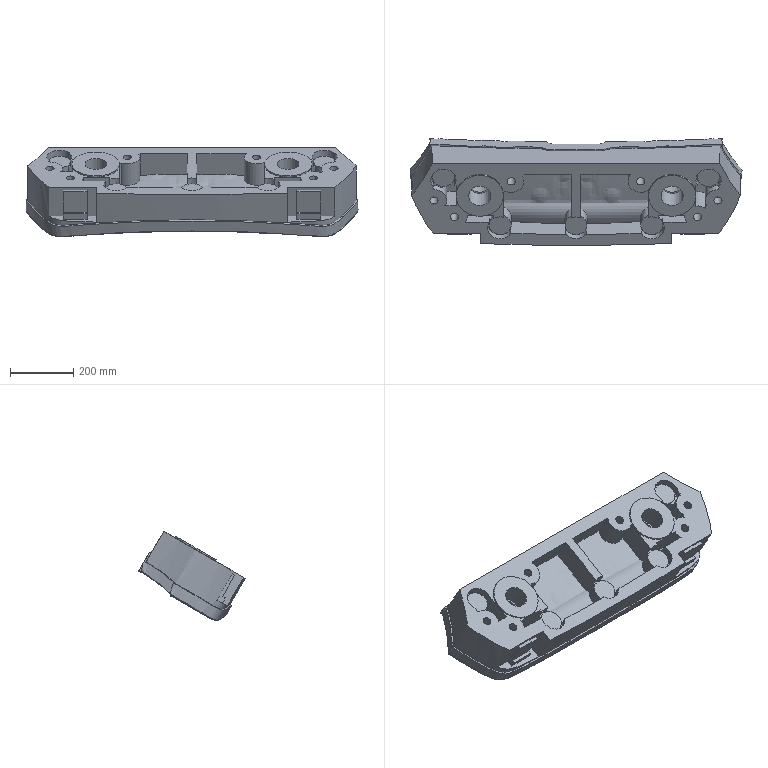Part | NX | features solid 2 | 1 solid | 373 faces | box 1052 x 337.624 x 283.118 mm | volume 27473011 mm3 | spline 259 | plane 76 | cylinder 38 | commonest cylinder face diameters 80 x15 70 x7 26 x6 40 x6 60 x2 150 x2